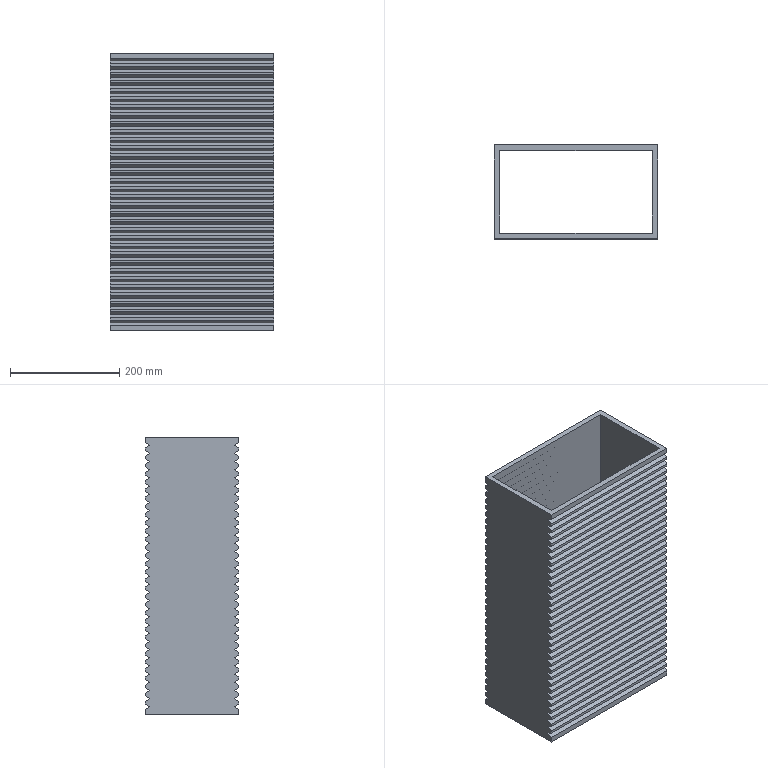Part | STEP file | Electric cylinder dust boot, cylinder C | 1 solid | 208 faces | box 300 x 172 x 510 mm | volume 3753035 mm3 | plane 208